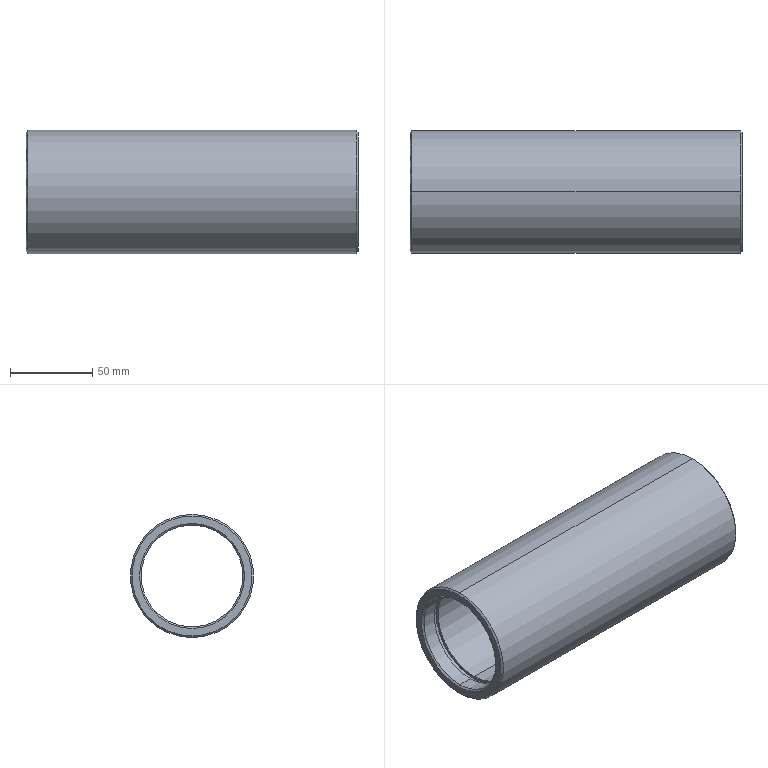Part | SolidWorks | features Chamfer 2, Revolution 1 | 1 solid | 30 faces | box 202 x 75 x 75 mm | volume 280318 mm3 | cone 12 | cylinder 12 | plane 6 | commonest cylinder face diameters 62 x6 65 x4 75 x2
STEP:
#1=CARTESIAN_POINT('',(9.126,0.,-31.));
#2=VERTEX_POINT('',#1);
#3=CARTESIAN_POINT('',(9.126,0.,31.));
#4=VERTEX_POINT('',#3);
#5=CARTESIAN_POINT('',(9.126,0.,0.));
#6=DIRECTION('',(-1.,0.,0.));
#7=DIRECTION('',(0.,0.,-1.));
#8=AXIS2_PLACEMENT_3D('',#5,#6,#7);
#9=CIRCLE('',#8,31.);
#10=EDGE_CURVE('',#2,#4,#9,.T.);
#11=ORIENTED_EDGE('',*,*,#10,.F.);
#12=CARTESIAN_POINT('',(8.876,0.,-31.25));
#13=VERTEX_POINT('',#12);
#14=CARTESIAN_POINT('',(9.126,0.,-31.));
#15=DIRECTION('',(-0.7071,0.,-0.7071));
#16=VECTOR('',#15,1000.);
#17=LINE('',#14,#16);
#18=EDGE_CURVE('',#2,#13,#17,.T.);
#19=ORIENTED_EDGE('',*,*,#18,.T.);
#20=CARTESIAN_POINT('',(8.876,0.,31.25));
#21=VERTEX_POINT('',#20);
#22=CARTESIAN_POINT('',(8.876,0.,0.));
#23=DIRECTION('',(1.,0.,0.));
#24=DIRECTION('',(0.,0.,-1.));
#25=AXIS2_PLACEMENT_3D('',#22,#23,#24);
#26=CIRCLE('',#25,31.25);
#27=EDGE_CURVE('',#21,#13,#26,.T.);
#28=ORIENTED_EDGE('',*,*,#27,.F.);
#29=CARTESIAN_POINT('',(9.126,0.,31.));
#30=DIRECTION('',(-0.7071,0.,0.7071));
#31=VECTOR('',#30,1000.);
#32=LINE('',#29,#31);
#33=EDGE_CURVE('',#4,#21,#32,.T.);
#34=ORIENTED_EDGE('',*,*,#33,.F.);
#35=EDGE_LOOP('',(#11,#19,#28,#34));
#36=FACE_OUTER_BOUND('',#35,.T.);
#37=CARTESIAN_POINT('',(9.126,0.,0.));
#38=DIRECTION('',(-1.,0.,0.));
#39=DIRECTION('',(0.,0.,1.));
#40=AXIS2_PLACEMENT_3D('',#37,#38,#39);
#41=CONICAL_SURFACE('',#40,31.,0.7854);
#42=ADVANCED_FACE('',(#36),#41,.F.);
#43=CARTESIAN_POINT('',(184.626,0.,31.));
#44=VERTEX_POINT('',#43);
#45=CARTESIAN_POINT('',(184.626,0.,-31.));
#46=VERTEX_POINT('',#45);
#47=CARTESIAN_POINT('',(184.626,0.,0.));
#48=DIRECTION('',(1.,0.,0.));
#49=DIRECTION('',(0.,0.,1.));
#50=AXIS2_PLACEMENT_3D('',#47,#48,#49);
#51=CIRCLE('',#50,31.);
#52=EDGE_CURVE('',#44,#46,#51,.T.);
#53=ORIENTED_EDGE('',*,*,#52,.F.);
#54=CARTESIAN_POINT('',(184.876,0.,31.25));
#55=VERTEX_POINT('',#54);
#56=CARTESIAN_POINT('',(184.876,0.,31.25));
#57=DIRECTION('',(0.7071,0.,0.7071));
#58=VECTOR('',#57,1000.);
#59=LINE('',#56,#58);
#60=EDGE_CURVE('',#44,#55,#59,.T.);
#61=ORIENTED_EDGE('',*,*,#60,.T.);
#62=CARTESIAN_POINT('',(184.876,0.,-31.25));
#63=VERTEX_POINT('',#62);
#64=CARTESIAN_POINT('',(184.876,0.,0.));
#65=DIRECTION('',(-1.,0.,0.));
#66=DIRECTION('',(0.,0.,1.));
#67=AXIS2_PLACEMENT_3D('',#64,#65,#66);
#68=CIRCLE('',#67,31.25);
#69=EDGE_CURVE('',#63,#55,#68,.T.);
#70=ORIENTED_EDGE('',*,*,#69,.F.);
#71=CARTESIAN_POINT('',(184.876,0.,-31.25));
#72=DIRECTION('',(0.7071,0.,-0.7071));
#73=VECTOR('',#72,1000.);
#74=LINE('',#71,#73);
#75=EDGE_CURVE('',#46,#63,#74,.T.);
#76=ORIENTED_EDGE('',*,*,#75,.F.);
#77=EDGE_LOOP('',(#53,#61,#70,#76));
#78=FACE_OUTER_BOUND('',#77,.T.);
#79=CARTESIAN_POINT('',(184.876,0.,0.));
#80=DIRECTION('',(1.,0.,0.));
#81=DIRECTION('',(0.,0.,-1.));
#82=AXIS2_PLACEMENT_3D('',#79,#80,#81);
#83=CONICAL_SURFACE('',#82,31.25,0.7854);
#84=ADVANCED_FACE('',(#78),#83,.F.);
#85=CARTESIAN_POINT('',(196.876,0.,31.));
#86=VERTEX_POINT('',#85);
#87=CARTESIAN_POINT('',(196.876,0.,-31.));
#88=VERTEX_POINT('',#87);
#89=CARTESIAN_POINT('',(196.876,0.,0.));
#90=DIRECTION('',(1.,0.,0.));
#91=DIRECTION('',(0.,0.,1.));
#92=AXIS2_PLACEMENT_3D('',#89,#90,#91);
#93=CIRCLE('',#92,31.);
#94=EDGE_CURVE('',#86,#88,#93,.T.);
#95=ORIENTED_EDGE('',*,*,#94,.F.);
#96=CARTESIAN_POINT('',(197.876,0.,32.));
#97=VERTEX_POINT('',#96);
#98=CARTESIAN_POINT('',(197.876,0.,32.));
#99=DIRECTION('',(0.7071,0.,0.7071));
#100=VECTOR('',#99,1000.);
#101=LINE('',#98,#100);
#102=EDGE_CURVE('',#86,#97,#101,.T.);
#103=ORIENTED_EDGE('',*,*,#102,.T.);
#104=CARTESIAN_POINT('',(197.876,0.,-32.));
#105=VERTEX_POINT('',#104);
#106=CARTESIAN_POINT('',(197.876,0.,0.));
#107=DIRECTION('',(-1.,0.,0.));
#108=DIRECTION('',(0.,0.,1.));
#109=AXIS2_PLACEMENT_3D('',#106,#107,#108);
#110=CIRCLE('',#109,32.);
#111=EDGE_CURVE('',#105,#97,#110,.T.);
#112=ORIENTED_EDGE('',*,*,#111,.F.);
#113=CARTESIAN_POINT('',(197.876,0.,-32.));
#114=DIRECTION('',(0.7071,0.,-0.7071));
#115=VECTOR('',#114,1000.);
#116=LINE('',#113,#115);
#117=EDGE_CURVE('',#88,#105,#116,.T.);
#118=ORIENTED_EDGE('',*,*,#117,.F.);
#119=EDGE_LOOP('',(#95,#103,#112,#118));
#120=FACE_OUTER_BOUND('',#119,.T.);
#121=CARTESIAN_POINT('',(197.876,0.,0.));
#122=DIRECTION('',(1.,0.,0.));
#123=DIRECTION('',(0.,0.,-1.));
#124=AXIS2_PLACEMENT_3D('',#121,#122,#123);
#125=CONICAL_SURFACE('',#124,32.,0.7854);
#126=ADVANCED_FACE('',(#120),#125,.F.);
#127=CARTESIAN_POINT('',(197.876,0.,-36.5));
#128=VERTEX_POINT('',#127);
#129=CARTESIAN_POINT('',(197.876,0.,36.5));
#130=VERTEX_POINT('',#129);
#131=CARTESIAN_POINT('',(197.876,0.,0.));
#132=DIRECTION('',(1.,0.,0.));
#133=DIRECTION('',(0.,0.,1.));
#134=AXIS2_PLACEMENT_3D('',#131,#132,#133);
#135=CIRCLE('',#134,36.5);
#136=EDGE_CURVE('',#128,#130,#135,.T.);
#137=ORIENTED_EDGE('',*,*,#136,.F.);
#138=CARTESIAN_POINT('',(196.876,0.,-37.5));
#139=VERTEX_POINT('',#138);
#140=CARTESIAN_POINT('',(196.876,0.,-37.5));
#141=DIRECTION('',(-0.7071,0.,-0.7071));
#142=VECTOR('',#141,1000.);
#143=LINE('',#140,#142);
#144=EDGE_CURVE('',#128,#139,#143,.T.);
#145=ORIENTED_EDGE('',*,*,#144,.T.);
#146=CARTESIAN_POINT('',(196.876,0.,37.5));
#147=VERTEX_POINT('',#146);
#148=CARTESIAN_POINT('',(196.876,0.,0.));
#149=DIRECTION('',(-1.,0.,0.));
#150=DIRECTION('',(0.,0.,1.));
#151=AXIS2_PLACEMENT_3D('',#148,#149,#150);
#152=CIRCLE('',#151,37.5);
#153=EDGE_CURVE('',#147,#139,#152,.T.);
#154=ORIENTED_EDGE('',*,*,#153,.F.);
#155=CARTESIAN_POINT('',(196.876,0.,37.5));
#156=DIRECTION('',(-0.7071,0.,0.7071));
#157=VECTOR('',#156,1000.);
#158=LINE('',#155,#157);
#159=EDGE_CURVE('',#130,#147,#158,.T.);
#160=ORIENTED_EDGE('',*,*,#159,.F.);
#161=EDGE_LOOP('',(#137,#145,#154,#160));
#162=FACE_OUTER_BOUND('',#161,.T.);
#163=CARTESIAN_POINT('',(196.876,0.,0.));
#164=DIRECTION('',(-1.,0.,0.));
#165=DIRECTION('',(0.,0.,1.));
#166=AXIS2_PLACEMENT_3D('',#163,#164,#165);
#167=CONICAL_SURFACE('',#166,37.5,0.7854);
#168=ADVANCED_FACE('',(#162),#167,.T.);
#169=CARTESIAN_POINT('',(-3.124,0.,-31.));
#170=VERTEX_POINT('',#169);
#171=CARTESIAN_POINT('',(-3.124,0.,31.));
#172=VERTEX_POINT('',#171);
#173=CARTESIAN_POINT('',(-3.124,0.,0.));
#174=DIRECTION('',(-1.,0.,0.));
#175=DIRECTION('',(0.,0.,-1.));
#176=AXIS2_PLACEMENT_3D('',#173,#174,#175);
#177=CIRCLE('',#176,31.);
#178=EDGE_CURVE('',#170,#172,#177,.T.);
#179=ORIENTED_EDGE('',*,*,#178,.F.);
#180=CARTESIAN_POINT('',(-4.124,0.,-32.));
#181=VERTEX_POINT('',#180);
#182=CARTESIAN_POINT('',(-3.124,0.,-31.));
#183=DIRECTION('',(-0.7071,0.,-0.7071));
#184=VECTOR('',#183,1000.);
#185=LINE('',#182,#184);
#186=EDGE_CURVE('',#170,#181,#185,.T.);
#187=ORIENTED_EDGE('',*,*,#186,.T.);
#188=CARTESIAN_POINT('',(-4.124,0.,32.));
#189=VERTEX_POINT('',#188);
#190=CARTESIAN_POINT('',(-4.124,0.,0.));
#191=DIRECTION('',(1.,0.,0.));
#192=DIRECTION('',(0.,0.,-1.));
#193=AXIS2_PLACEMENT_3D('',#190,#191,#192);
#194=CIRCLE('',#193,32.);
#195=EDGE_CURVE('',#189,#181,#194,.T.);
#196=ORIENTED_EDGE('',*,*,#195,.F.);
#197=CARTESIAN_POINT('',(-3.124,0.,31.));
#198=DIRECTION('',(-0.7071,0.,0.7071));
#199=VECTOR('',#198,1000.);
#200=LINE('',#197,#199);
#201=EDGE_CURVE('',#172,#189,#200,.T.);
#202=ORIENTED_EDGE('',*,*,#201,.F.);
#203=EDGE_LOOP('',(#179,#187,#196,#202));
#204=FACE_OUTER_BOUND('',#203,.T.);
#205=CARTESIAN_POINT('',(-3.124,0.,0.));
#206=DIRECTION('',(-1.,0.,0.));
#207=DIRECTION('',(0.,0.,1.));
#208=AXIS2_PLACEMENT_3D('',#205,#206,#207);
#209=CONICAL_SURFACE('',#208,31.,0.7854);
#210=ADVANCED_FACE('',(#204),#209,.F.);
#211=CARTESIAN_POINT('',(-4.124,0.,36.5));
#212=VERTEX_POINT('',#211);
#213=CARTESIAN_POINT('',(-4.124,0.,-36.5));
#214=VERTEX_POINT('',#213);
#215=CARTESIAN_POINT('',(-4.124,0.,0.));
#216=DIRECTION('',(-1.,0.,0.));
#217=DIRECTION('',(0.,0.,-1.));
#218=AXIS2_PLACEMENT_3D('',#215,#216,#217);
#219=CIRCLE('',#218,36.5);
#220=EDGE_CURVE('',#212,#214,#219,.T.);
#221=ORIENTED_EDGE('',*,*,#220,.F.);
#222=CARTESIAN_POINT('',(-3.124,0.,37.5));
#223=VERTEX_POINT('',#222);
#224=CARTESIAN_POINT('',(-4.124,0.,36.5));
#225=DIRECTION('',(0.7071,0.,0.7071));
#226=VECTOR('',#225,1000.);
#227=LINE('',#224,#226);
#228=EDGE_CURVE('',#212,#223,#227,.T.);
#229=ORIENTED_EDGE('',*,*,#228,.T.);
#230=CARTESIAN_POINT('',(-3.124,0.,-37.5));
#231=VERTEX_POINT('',#230);
#232=CARTESIAN_POINT('',(-3.124,0.,0.));
#233=DIRECTION('',(1.,0.,0.));
#234=DIRECTION('',(0.,0.,-1.));
#235=AXIS2_PLACEMENT_3D('',#232,#233,#234);
#236=CIRCLE('',#235,37.5);
#237=EDGE_CURVE('',#231,#223,#236,.T.);
#238=ORIENTED_EDGE('',*,*,#237,.F.);
#239=CARTESIAN_POINT('',(-4.124,0.,-36.5));
#240=DIRECTION('',(0.7071,0.,-0.7071));
#241=VECTOR('',#240,1000.);
#242=LINE('',#239,#241);
#243=EDGE_CURVE('',#214,#231,#242,.T.);
#244=ORIENTED_EDGE('',*,*,#243,.F.);
#245=EDGE_LOOP('',(#221,#229,#238,#244));
#246=FACE_OUTER_BOUND('',#245,.T.);
#247=CARTESIAN_POINT('',(-4.124,0.,0.));
#248=DIRECTION('',(1.,0.,0.));
#249=DIRECTION('',(0.,0.,-1.));
#250=AXIS2_PLACEMENT_3D('',#247,#248,#249);
#251=CONICAL_SURFACE('',#250,36.5,0.7854);
#252=ADVANCED_FACE('',(#246),#251,.T.);
#253=CARTESIAN_POINT('',(5.876,0.,-31.));
#254=VERTEX_POINT('',#253);
#255=CARTESIAN_POINT('',(5.876,0.,31.));
#256=VERTEX_POINT('',#255);
#257=CARTESIAN_POINT('',(5.876,0.,0.));
#258=DIRECTION('',(-1.,0.,0.));
#259=DIRECTION('',(0.,0.,1.));
#260=AXIS2_PLACEMENT_3D('',#257,#258,#259);
#261=CIRCLE('',#260,31.);
#262=EDGE_CURVE('',#254,#256,#261,.T.);
#263=ORIENTED_EDGE('',*,*,#262,.F.);
#264=CARTESIAN_POINT('',(0.,0.,-31.));
#265=DIRECTION('',(-1.,0.,0.));
#266=VECTOR('',#265,1000.);
#267=LINE('',#264,#266);
#268=EDGE_CURVE('',#254,#170,#267,.T.);
#269=ORIENTED_EDGE('',*,*,#268,.T.);
#270=ORIENTED_EDGE('',*,*,#178,.T.);
#271=CARTESIAN_POINT('',(0.,0.,31.));
#272=DIRECTION('',(-1.,0.,0.));
#273=VECTOR('',#272,1000.);
#274=LINE('',#271,#273);
#275=EDGE_CURVE('',#256,#172,#274,.T.);
#276=ORIENTED_EDGE('',*,*,#275,.F.);
#277=EDGE_LOOP('',(#263,#269,#270,#276));
#278=FACE_OUTER_BOUND('',#277,.T.);
#279=CARTESIAN_POINT('',(0.,0.,0.));
#280=DIRECTION('',(-1.,0.,0.));
#281=DIRECTION('',(0.,0.,1.));
#282=AXIS2_PLACEMENT_3D('',#279,#280,#281);
#283=CYLINDRICAL_SURFACE('',#282,31.);
#284=ADVANCED_FACE('',(#278),#283,.F.);
#285=CARTESIAN_POINT('',(8.876,0.,-32.5));
#286=VERTEX_POINT('',#285);
#287=CARTESIAN_POINT('',(8.876,0.,32.5));
#288=VERTEX_POINT('',#287);
#289=CARTESIAN_POINT('',(8.876,0.,0.));
#290=DIRECTION('',(-1.,0.,0.));
#291=DIRECTION('',(0.,0.,1.));
#292=AXIS2_PLACEMENT_3D('',#289,#290,#291);
#293=CIRCLE('',#292,32.5);
#294=EDGE_CURVE('',#286,#288,#293,.T.);
#295=ORIENTED_EDGE('',*,*,#294,.F.);
#296=CARTESIAN_POINT('',(5.876,0.,-32.5));
#297=VERTEX_POINT('',#296);
#298=CARTESIAN_POINT('',(0.,0.,-32.5));
#299=DIRECTION('',(-1.,0.,0.));
#300=VECTOR('',#299,1000.);
#301=LINE('',#298,#300);
#302=EDGE_CURVE('',#286,#297,#301,.T.);
#303=ORIENTED_EDGE('',*,*,#302,.T.);
#304=CARTESIAN_POINT('',(5.876,0.,32.5));
#305=VERTEX_POINT('',#304);
#306=CARTESIAN_POINT('',(5.876,0.,0.));
#307=DIRECTION('',(-1.,0.,0.));
#308=DIRECTION('',(0.,0.,1.));
#309=AXIS2_PLACEMENT_3D('',#306,#307,#308);
#310=CIRCLE('',#309,32.5);
#311=EDGE_CURVE('',#297,#305,#310,.T.);
#312=ORIENTED_EDGE('',*,*,#311,.T.);
#313=CARTESIAN_POINT('',(0.,0.,32.5));
#314=DIRECTION('',(-1.,0.,0.));
#315=VECTOR('',#314,1000.);
#316=LINE('',#313,#315);
#317=EDGE_CURVE('',#288,#305,#316,.T.);
#318=ORIENTED_EDGE('',*,*,#317,.F.);
#319=EDGE_LOOP('',(#295,#303,#312,#318));
#320=FACE_OUTER_BOUND('',#319,.T.);
#321=CARTESIAN_POINT('',(0.,0.,0.));
#322=DIRECTION('',(-1.,0.,0.));
#323=DIRECTION('',(0.,0.,1.));
#324=AXIS2_PLACEMENT_3D('',#321,#322,#323);
#325=CYLINDRICAL_SURFACE('',#324,32.5);
#326=ADVANCED_FACE('',(#320),#325,.F.);
#327=ORIENTED_EDGE('',*,*,#52,.T.);
#328=CARTESIAN_POINT('',(0.,0.,-31.));
#329=DIRECTION('',(-1.,0.,0.));
#330=VECTOR('',#329,1000.);
#331=LINE('',#328,#330);
#332=EDGE_CURVE('',#46,#2,#331,.T.);
#333=ORIENTED_EDGE('',*,*,#332,.T.);
#334=ORIENTED_EDGE('',*,*,#10,.T.);
#335=CARTESIAN_POINT('',(0.,0.,31.));
#336=DIRECTION('',(-1.,0.,0.));
#337=VECTOR('',#336,1000.);
#338=LINE('',#335,#337);
#339=EDGE_CURVE('',#44,#4,#338,.T.);
#340=ORIENTED_EDGE('',*,*,#339,.F.);
#341=EDGE_LOOP('',(#327,#333,#334,#340));
#342=FACE_OUTER_BOUND('',#341,.T.);
#343=CARTESIAN_POINT('',(0.,0.,0.));
#344=DIRECTION('',(-1.,0.,0.));
#345=DIRECTION('',(0.,0.,1.));
#346=AXIS2_PLACEMENT_3D('',#343,#344,#345);
#347=CYLINDRICAL_SURFACE('',#346,31.);
#348=ADVANCED_FACE('',(#342),#347,.F.);
#349=CARTESIAN_POINT('',(187.876,0.,-32.5));
#350=VERTEX_POINT('',#349);
#351=CARTESIAN_POINT('',(187.876,0.,32.5));
#352=VERTEX_POINT('',#351);
#353=CARTESIAN_POINT('',(187.876,0.,0.));
#354=DIRECTION('',(-1.,0.,0.));
#355=DIRECTION('',(0.,0.,1.));
#356=AXIS2_PLACEMENT_3D('',#353,#354,#355);
#357=CIRCLE('',#356,32.5);
#358=EDGE_CURVE('',#350,#352,#357,.T.);
#359=ORIENTED_EDGE('',*,*,#358,.F.);
#360=CARTESIAN_POINT('',(184.876,0.,-32.5));
#361=VERTEX_POINT('',#360);
#362=CARTESIAN_POINT('',(0.,0.,-32.5));
#363=DIRECTION('',(-1.,0.,0.));
#364=VECTOR('',#363,1000.);
#365=LINE('',#362,#364);
#366=EDGE_CURVE('',#350,#361,#365,.T.);
#367=ORIENTED_EDGE('',*,*,#366,.T.);
#368=CARTESIAN_POINT('',(184.876,0.,32.5));
#369=VERTEX_POINT('',#368);
#370=CARTESIAN_POINT('',(184.876,0.,0.));
#371=DIRECTION('',(-1.,0.,0.));
#372=DIRECTION('',(0.,0.,1.));
#373=AXIS2_PLACEMENT_3D('',#370,#371,#372);
#374=CIRCLE('',#373,32.5);
#375=EDGE_CURVE('',#361,#369,#374,.T.);
#376=ORIENTED_EDGE('',*,*,#375,.T.);
#377=CARTESIAN_POINT('',(0.,0.,32.5));
#378=DIRECTION('',(-1.,0.,0.));
#379=VECTOR('',#378,1000.);
#380=LINE('',#377,#379);
#381=EDGE_CURVE('',#352,#369,#380,.T.);
#382=ORIENTED_EDGE('',*,*,#381,.F.);
#383=EDGE_LOOP('',(#359,#367,#376,#382));
#384=FACE_OUTER_BOUND('',#383,.T.);
#385=CARTESIAN_POINT('',(0.,0.,0.));
#386=DIRECTION('',(-1.,0.,0.));
#387=DIRECTION('',(0.,0.,1.));
#388=AXIS2_PLACEMENT_3D('',#385,#386,#387);
#389=CYLINDRICAL_SURFACE('',#388,32.5);
#390=ADVANCED_FACE('',(#384),#389,.F.);
#391=ORIENTED_EDGE('',*,*,#94,.T.);
#392=CARTESIAN_POINT('',(187.876,0.,-31.));
#393=VERTEX_POINT('',#392);
#394=CARTESIAN_POINT('',(0.,0.,-31.));
#395=DIRECTION('',(-1.,0.,0.));
#396=VECTOR('',#395,1000.);
#397=LINE('',#394,#396);
#398=EDGE_CURVE('',#88,#393,#397,.T.);
#399=ORIENTED_EDGE('',*,*,#398,.T.);
#400=CARTESIAN_POINT('',(187.876,0.,31.));
#401=VERTEX_POINT('',#400);
#402=CARTESIAN_POINT('',(187.876,0.,0.));
#403=DIRECTION('',(-1.,0.,0.));
#404=DIRECTION('',(0.,0.,1.));
#405=AXIS2_PLACEMENT_3D('',#402,#403,#404);
#406=CIRCLE('',#405,31.);
#407=EDGE_CURVE('',#393,#401,#406,.T.);
#408=ORIENTED_EDGE('',*,*,#407,.T.);
#409=CARTESIAN_POINT('',(0.,0.,31.));
#410=DIRECTION('',(-1.,0.,0.));
#411=VECTOR('',#410,1000.);
#412=LINE('',#409,#411);
#413=EDGE_CURVE('',#86,#401,#412,.T.);
#414=ORIENTED_EDGE('',*,*,#413,.F.);
#415=EDGE_LOOP('',(#391,#399,#408,#414));
#416=FACE_OUTER_BOUND('',#415,.T.);
#417=CARTESIAN_POINT('',(0.,0.,0.));
#418=DIRECTION('',(-1.,0.,0.));
#419=DIRECTION('',(0.,0.,1.));
#420=AXIS2_PLACEMENT_3D('',#417,#418,#419);
#421=CYLINDRICAL_SURFACE('',#420,31.);
#422=ADVANCED_FACE('',(#416),#421,.F.);
#423=ORIENTED_EDGE('',*,*,#153,.T.);
#424=CARTESIAN_POINT('',(0.,0.,-37.5));
#425=DIRECTION('',(-1.,0.,0.));
#426=VECTOR('',#425,1000.);
#427=LINE('',#424,#426);
#428=EDGE_CURVE('',#139,#231,#427,.T.);
#429=ORIENTED_EDGE('',*,*,#428,.T.);
#430=ORIENTED_EDGE('',*,*,#237,.T.);
#431=CARTESIAN_POINT('',(0.,0.,37.5));
#432=DIRECTION('',(-1.,0.,0.));
#433=VECTOR('',#432,1000.);
#434=LINE('',#431,#433);
#435=EDGE_CURVE('',#147,#223,#434,.T.);
#436=ORIENTED_EDGE('',*,*,#435,.F.);
#437=EDGE_LOOP('',(#423,#429,#430,#436));
#438=FACE_OUTER_BOUND('',#437,.T.);
#439=CARTESIAN_POINT('',(0.,0.,0.));
#440=DIRECTION('',(-1.,0.,0.));
#441=DIRECTION('',(0.,0.,1.));
#442=AXIS2_PLACEMENT_3D('',#439,#440,#441);
#443=CYLINDRICAL_SURFACE('',#442,37.5);
#444=ADVANCED_FACE('',(#438),#443,.T.);
#445=CARTESIAN_POINT('',(-4.124,0.,0.));
#446=DIRECTION('',(-1.,0.,0.));
#447=DIRECTION('',(0.,0.,-1.));
#448=AXIS2_PLACEMENT_3D('',#445,#446,#447);
#449=CIRCLE('',#448,36.5);
#450=EDGE_CURVE('',#214,#212,#449,.T.);
#451=ORIENTED_EDGE('',*,*,#450,.T.);
#452=ORIENTED_EDGE('',*,*,#220,.T.);
#453=EDGE_LOOP('',(#451,#452));
#454=FACE_OUTER_BOUND('',#453,.T.);
#455=ORIENTED_EDGE('',*,*,#195,.T.);
#456=CARTESIAN_POINT('',(-4.124,0.,0.));
#457=DIRECTION('',(1.,0.,0.));
#458=DIRECTION('',(0.,0.,-1.));
#459=AXIS2_PLACEMENT_3D('',#456,#457,#458);
#460=CIRCLE('',#459,32.);
#461=EDGE_CURVE('',#181,#189,#460,.T.);
#462=ORIENTED_EDGE('',*,*,#461,.T.);
#463=EDGE_LOOP('',(#455,#462));
#464=FACE_BOUND('',#463,.T.);
#465=CARTESIAN_POINT('',(-4.124,31.,0.));
#466=DIRECTION('',(1.,0.,0.));
#467=DIRECTION('',(0.,0.,-1.));
#468=AXIS2_PLACEMENT_3D('',#465,#466,#467);
#469=PLANE('',#468);
#470=ADVANCED_FACE('',(#454,#464),#469,.F.);
#471=ORIENTED_EDGE('',*,*,#428,.F.);
#472=CARTESIAN_POINT('',(196.876,0.,0.));
#473=DIRECTION('',(-1.,0.,0.));
#474=DIRECTION('',(0.,0.,1.));
#475=AXIS2_PLACEMENT_3D('',#472,#473,#474);
#476=CIRCLE('',#475,37.5);
#477=EDGE_CURVE('',#139,#147,#476,.T.);
#478=ORIENTED_EDGE('',*,*,#477,.T.);
#479=ORIENTED_EDGE('',*,*,#435,.T.);
#480=CARTESIAN_POINT('',(-3.124,0.,0.));
#481=DIRECTION('',(1.,0.,0.));
#482=DIRECTION('',(0.,0.,-1.));
#483=AXIS2_PLACEMENT_3D('',#480,#481,#482);
#484=CIRCLE('',#483,37.5);
#485=EDGE_CURVE('',#223,#231,#484,.T.);
#486=ORIENTED_EDGE('',*,*,#485,.T.);
#487=EDGE_LOOP('',(#471,#478,#479,#486));
#488=FACE_OUTER_BOUND('',#487,.T.);
#489=CARTESIAN_POINT('',(0.,0.,0.));
#490=DIRECTION('',(-1.,0.,0.));
#491=DIRECTION('',(0.,0.,1.));
#492=AXIS2_PLACEMENT_3D('',#489,#490,#491);
#493=CYLINDRICAL_SURFACE('',#492,37.5);
#494=ADVANCED_FACE('',(#488),#493,.T.);
#495=CARTESIAN_POINT('',(197.876,0.,0.));
#496=DIRECTION('',(1.,0.,0.));
#497=DIRECTION('',(0.,0.,1.));
#498=AXIS2_PLACEMENT_3D('',#495,#496,#497);
#499=CIRCLE('',#498,36.5);
#500=EDGE_CURVE('',#130,#128,#499,.T.);
#501=ORIENTED_EDGE('',*,*,#500,.T.);
#502=ORIENTED_EDGE('',*,*,#136,.T.);
#503=EDGE_LOOP('',(#501,#502));
#504=FACE_OUTER_BOUND('',#503,.T.);
#505=ORIENTED_EDGE('',*,*,#111,.T.);
#506=CARTESIAN_POINT('',(197.876,0.,0.));
#507=DIRECTION('',(-1.,0.,0.));
#508=DIRECTION('',(0.,0.,1.));
#509=AXIS2_PLACEMENT_3D('',#506,#507,#508);
#510=CIRCLE('',#509,32.);
#511=EDGE_CURVE('',#97,#105,#510,.T.);
#512=ORIENTED_EDGE('',*,*,#511,.T.);
#513=EDGE_LOOP('',(#505,#512));
#514=FACE_BOUND('',#513,.T.);
#515=CARTESIAN_POINT('',(197.876,37.5,0.));
#516=DIRECTION('',(-1.,0.,0.));
#517=DIRECTION('',(0.,0.,1.));
#518=AXIS2_PLACEMENT_3D('',#515,#516,#517);
#519=PLANE('',#518);
#520=ADVANCED_FACE('',(#504,#514),#519,.F.);
#521=ORIENTED_EDGE('',*,*,#398,.F.);
#522=CARTESIAN_POINT('',(196.876,0.,0.));
#523=DIRECTION('',(1.,0.,0.));
#524=DIRECTION('',(0.,0.,1.));
#525=AXIS2_PLACEMENT_3D('',#522,#523,#524);
#526=CIRCLE('',#525,31.);
#527=EDGE_CURVE('',#88,#86,#526,.T.);
#528=ORIENTED_EDGE('',*,*,#527,.T.);
#529=ORIENTED_EDGE('',*,*,#413,.T.);
#530=CARTESIAN_POINT('',(187.876,0.,0.));
#531=DIRECTION('',(-1.,0.,0.));
#532=DIRECTION('',(0.,0.,1.));
#533=AXIS2_PLACEMENT_3D('',#530,#531,#532);
#534=CIRCLE('',#533,31.);
#535=EDGE_CURVE('',#401,#393,#534,.T.);
#536=ORIENTED_EDGE('',*,*,#535,.T.);
#537=EDGE_LOOP('',(#521,#528,#529,#536));
#538=FACE_OUTER_BOUND('',#537,.T.);
#539=CARTESIAN_POINT('',(0.,0.,0.));
#540=DIRECTION('',(-1.,0.,0.));
#541=DIRECTION('',(0.,0.,1.));
#542=AXIS2_PLACEMENT_3D('',#539,#540,#541);
#543=CYLINDRICAL_SURFACE('',#542,31.);
#544=ADVANCED_FACE('',(#538),#543,.F.);
#545=ORIENTED_EDGE('',*,*,#535,.F.);
#546=ORIENTED_EDGE('',*,*,#407,.F.);
#547=EDGE_LOOP('',(#545,#546));
#548=FACE_BOUND('',#547,.T.);
#549=CARTESIAN_POINT('',(187.876,0.,0.));
#550=DIRECTION('',(-1.,0.,0.));
#551=DIRECTION('',(0.,0.,1.));
#552=AXIS2_PLACEMENT_3D('',#549,#550,#551);
#553=CIRCLE('',#552,32.5);
#554=EDGE_CURVE('',#352,#350,#553,.T.);
#555=ORIENTED_EDGE('',*,*,#554,.T.);
#556=ORIENTED_EDGE('',*,*,#358,.T.);
#557=EDGE_LOOP('',(#555,#556));
#558=FACE_OUTER_BOUND('',#557,.T.);
#559=CARTESIAN_POINT('',(187.876,31.,0.));
#560=DIRECTION('',(1.,0.,0.));
#561=DIRECTION('',(0.,0.,-1.));
#562=AXIS2_PLACEMENT_3D('',#559,#560,#561);
#563=PLANE('',#562);
#564=ADVANCED_FACE('',(#548,#558),#563,.F.);
#565=ORIENTED_EDGE('',*,*,#366,.F.);
#566=ORIENTED_EDGE('',*,*,#554,.F.);
#567=ORIENTED_EDGE('',*,*,#381,.T.);
#568=CARTESIAN_POINT('',(184.876,0.,0.));
#569=DIRECTION('',(-1.,0.,0.));
#570=DIRECTION('',(0.,0.,1.));
#571=AXIS2_PLACEMENT_3D('',#568,#569,#570);
#572=CIRCLE('',#571,32.5);
#573=EDGE_CURVE('',#369,#361,#572,.T.);
#574=ORIENTED_EDGE('',*,*,#573,.T.);
#575=EDGE_LOOP('',(#565,#566,#567,#574));
#576=FACE_OUTER_BOUND('',#575,.T.);
#577=CARTESIAN_POINT('',(0.,0.,0.));
#578=DIRECTION('',(-1.,0.,0.));
#579=DIRECTION('',(0.,0.,1.));
#580=AXIS2_PLACEMENT_3D('',#577,#578,#579);
#581=CYLINDRICAL_SURFACE('',#580,32.5);
#582=ADVANCED_FACE('',(#576),#581,.F.);
#583=ORIENTED_EDGE('',*,*,#69,.T.);
#584=CARTESIAN_POINT('',(184.876,0.,0.));
#585=DIRECTION('',(-1.,0.,0.));
#586=DIRECTION('',(0.,0.,1.));
#587=AXIS2_PLACEMENT_3D('',#584,#585,#586);
#588=CIRCLE('',#587,31.25);
#589=EDGE_CURVE('',#55,#63,#588,.T.);
#590=ORIENTED_EDGE('',*,*,#589,.T.);
#591=EDGE_LOOP('',(#583,#590));
#592=FACE_BOUND('',#591,.T.);
#593=ORIENTED_EDGE('',*,*,#573,.F.);
#594=ORIENTED_EDGE('',*,*,#375,.F.);
#595=EDGE_LOOP('',(#593,#594));
#596=FACE_OUTER_BOUND('',#595,.T.);
#597=CARTESIAN_POINT('',(184.876,32.5,0.));
#598=DIRECTION('',(-1.,0.,0.));
#599=DIRECTION('',(0.,0.,1.));
#600=AXIS2_PLACEMENT_3D('',#597,#598,#599);
#601=PLANE('',#600);
#602=ADVANCED_FACE('',(#592,#596),#601,.F.);
#603=ORIENTED_EDGE('',*,*,#332,.F.);
#604=CARTESIAN_POINT('',(184.626,0.,0.));
#605=DIRECTION('',(1.,0.,0.));
#606=DIRECTION('',(0.,0.,1.));
#607=AXIS2_PLACEMENT_3D('',#604,#605,#606);
#608=CIRCLE('',#607,31.);
#609=EDGE_CURVE('',#46,#44,#608,.T.);
#610=ORIENTED_EDGE('',*,*,#609,.T.);
#611=ORIENTED_EDGE('',*,*,#339,.T.);
#612=CARTESIAN_POINT('',(9.126,0.,0.));
#613=DIRECTION('',(-1.,0.,0.));
#614=DIRECTION('',(0.,0.,-1.));
#615=AXIS2_PLACEMENT_3D('',#612,#613,#614);
#616=CIRCLE('',#615,31.);
#617=EDGE_CURVE('',#4,#2,#616,.T.);
#618=ORIENTED_EDGE('',*,*,#617,.T.);
#619=EDGE_LOOP('',(#603,#610,#611,#618));
#620=FACE_OUTER_BOUND('',#619,.T.);
#621=CARTESIAN_POINT('',(0.,0.,0.));
#622=DIRECTION('',(-1.,0.,0.));
#623=DIRECTION('',(0.,0.,1.));
#624=AXIS2_PLACEMENT_3D('',#621,#622,#623);
#625=CYLINDRICAL_SURFACE('',#624,31.);
#626=ADVANCED_FACE('',(#620),#625,.F.);
#627=ORIENTED_EDGE('',*,*,#27,.T.);
#628=CARTESIAN_POINT('',(8.876,0.,0.));
#629=DIRECTION('',(1.,0.,0.));
#630=DIRECTION('',(0.,0.,-1.));
#631=AXIS2_PLACEMENT_3D('',#628,#629,#630);
#632=CIRCLE('',#631,31.25);
#633=EDGE_CURVE('',#13,#21,#632,.T.);
#634=ORIENTED_EDGE('',*,*,#633,.T.);
#635=EDGE_LOOP('',(#627,#634));
#636=FACE_BOUND('',#635,.T.);
#637=CARTESIAN_POINT('',(8.876,0.,0.));
#638=DIRECTION('',(-1.,0.,0.));
#639=DIRECTION('',(0.,0.,1.));
#640=AXIS2_PLACEMENT_3D('',#637,#638,#639);
#641=CIRCLE('',#640,32.5);
#642=EDGE_CURVE('',#288,#286,#641,.T.);
#643=ORIENTED_EDGE('',*,*,#642,.T.);
#644=ORIENTED_EDGE('',*,*,#294,.T.);
#645=EDGE_LOOP('',(#643,#644));
#646=FACE_OUTER_BOUND('',#645,.T.);
#647=CARTESIAN_POINT('',(8.876,32.5,0.));
#648=DIRECTION('',(1.,0.,0.));
#649=DIRECTION('',(0.,0.,-1.));
#650=AXIS2_PLACEMENT_3D('',#647,#648,#649);
#651=PLANE('',#650);
#652=ADVANCED_FACE('',(#636,#646),#651,.F.);
#653=ORIENTED_EDGE('',*,*,#302,.F.);
#654=ORIENTED_EDGE('',*,*,#642,.F.);
#655=ORIENTED_EDGE('',*,*,#317,.T.);
#656=CARTESIAN_POINT('',(5.876,0.,0.));
#657=DIRECTION('',(-1.,0.,0.));
#658=DIRECTION('',(0.,0.,1.));
#659=AXIS2_PLACEMENT_3D('',#656,#657,#658);
#660=CIRCLE('',#659,32.5);
#661=EDGE_CURVE('',#305,#297,#660,.T.);
#662=ORIENTED_EDGE('',*,*,#661,.T.);
#663=EDGE_LOOP('',(#653,#654,#655,#662));
#664=FACE_OUTER_BOUND('',#663,.T.);
#665=CARTESIAN_POINT('',(0.,0.,0.));
#666=DIRECTION('',(-1.,0.,0.));
#667=DIRECTION('',(0.,0.,1.));
#668=AXIS2_PLACEMENT_3D('',#665,#666,#667);
#669=CYLINDRICAL_SURFACE('',#668,32.5);
#670=ADVANCED_FACE('',(#664),#669,.F.);
#671=ORIENTED_EDGE('',*,*,#661,.F.);
#672=ORIENTED_EDGE('',*,*,#311,.F.);
#673=EDGE_LOOP('',(#671,#672));
#674=FACE_OUTER_BOUND('',#673,.T.);
#675=CARTESIAN_POINT('',(5.876,0.,0.));
#676=DIRECTION('',(-1.,0.,0.));
#677=DIRECTION('',(0.,0.,1.));
#678=AXIS2_PLACEMENT_3D('',#675,#676,#677);
#679=CIRCLE('',#678,31.);
#680=EDGE_CURVE('',#256,#254,#679,.T.);
#681=ORIENTED_EDGE('',*,*,#680,.T.);
#682=ORIENTED_EDGE('',*,*,#262,.T.);
#683=EDGE_LOOP('',(#681,#682));
#684=FACE_BOUND('',#683,.T.);
#685=CARTESIAN_POINT('',(5.876,31.,0.));
#686=DIRECTION('',(-1.,0.,0.));
#687=DIRECTION('',(0.,0.,1.));
#688=AXIS2_PLACEMENT_3D('',#685,#686,#687);
#689=PLANE('',#688);
#690=ADVANCED_FACE('',(#674,#684),#689,.F.);
#691=ORIENTED_EDGE('',*,*,#268,.F.);
#692=ORIENTED_EDGE('',*,*,#680,.F.);
#693=ORIENTED_EDGE('',*,*,#275,.T.);
#694=CARTESIAN_POINT('',(-3.124,0.,0.));
#695=DIRECTION('',(-1.,0.,0.));
#696=DIRECTION('',(0.,0.,-1.));
#697=AXIS2_PLACEMENT_3D('',#694,#695,#696);
#698=CIRCLE('',#697,31.);
#699=EDGE_CURVE('',#172,#170,#698,.T.);
#700=ORIENTED_EDGE('',*,*,#699,.T.);
#701=EDGE_LOOP('',(#691,#692,#693,#700));
#702=FACE_OUTER_BOUND('',#701,.T.);
#703=CARTESIAN_POINT('',(0.,0.,0.));
#704=DIRECTION('',(-1.,0.,0.));
#705=DIRECTION('',(0.,0.,1.));
#706=AXIS2_PLACEMENT_3D('',#703,#704,#705);
#707=CYLINDRICAL_SURFACE('',#706,31.);
#708=ADVANCED_FACE('',(#702),#707,.F.);
#709=ORIENTED_EDGE('',*,*,#228,.F.);
#710=ORIENTED_EDGE('',*,*,#450,.F.);
#711=ORIENTED_EDGE('',*,*,#243,.T.);
#712=ORIENTED_EDGE('',*,*,#485,.F.);
#713=EDGE_LOOP('',(#709,#710,#711,#712));
#714=FACE_OUTER_BOUND('',#713,.T.);
#715=CARTESIAN_POINT('',(-4.124,0.,0.));
#716=DIRECTION('',(1.,0.,0.));
#717=DIRECTION('',(0.,0.,-1.));
#718=AXIS2_PLACEMENT_3D('',#715,#716,#717);
#719=CONICAL_SURFACE('',#718,36.5,0.7854);
#720=ADVANCED_FACE('',(#714),#719,.T.);
#721=ORIENTED_EDGE('',*,*,#186,.F.);
#722=ORIENTED_EDGE('',*,*,#699,.F.);
#723=ORIENTED_EDGE('',*,*,#201,.T.);
#724=ORIENTED_EDGE('',*,*,#461,.F.);
#725=EDGE_LOOP('',(#721,#722,#723,#724));
#726=FACE_OUTER_BOUND('',#725,.T.);
#727=CARTESIAN_POINT('',(-3.124,0.,0.));
#728=DIRECTION('',(-1.,0.,0.));
#729=DIRECTION('',(0.,0.,1.));
#730=AXIS2_PLACEMENT_3D('',#727,#728,#729);
#731=CONICAL_SURFACE('',#730,31.,0.7854);
#732=ADVANCED_FACE('',(#726),#731,.F.);
#733=ORIENTED_EDGE('',*,*,#144,.F.);
#734=ORIENTED_EDGE('',*,*,#500,.F.);
#735=ORIENTED_EDGE('',*,*,#159,.T.);
#736=ORIENTED_EDGE('',*,*,#477,.F.);
#737=EDGE_LOOP('',(#733,#734,#735,#736));
#738=FACE_OUTER_BOUND('',#737,.T.);
#739=CARTESIAN_POINT('',(196.876,0.,0.));
#740=DIRECTION('',(-1.,0.,0.));
#741=DIRECTION('',(0.,0.,1.));
#742=AXIS2_PLACEMENT_3D('',#739,#740,#741);
#743=CONICAL_SURFACE('',#742,37.5,0.7854);
#744=ADVANCED_FACE('',(#738),#743,.T.);
#745=ORIENTED_EDGE('',*,*,#102,.F.);
#746=ORIENTED_EDGE('',*,*,#527,.F.);
#747=ORIENTED_EDGE('',*,*,#117,.T.);
#748=ORIENTED_EDGE('',*,*,#511,.F.);
#749=EDGE_LOOP('',(#745,#746,#747,#748));
#750=FACE_OUTER_BOUND('',#749,.T.);
#751=CARTESIAN_POINT('',(197.876,0.,0.));
#752=DIRECTION('',(1.,0.,0.));
#753=DIRECTION('',(0.,0.,-1.));
#754=AXIS2_PLACEMENT_3D('',#751,#752,#753);
#755=CONICAL_SURFACE('',#754,32.,0.7854);
#756=ADVANCED_FACE('',(#750),#755,.F.);
#757=ORIENTED_EDGE('',*,*,#60,.F.);
#758=ORIENTED_EDGE('',*,*,#609,.F.);
#759=ORIENTED_EDGE('',*,*,#75,.T.);
#760=ORIENTED_EDGE('',*,*,#589,.F.);
#761=EDGE_LOOP('',(#757,#758,#759,#760));
#762=FACE_OUTER_BOUND('',#761,.T.);
#763=CARTESIAN_POINT('',(184.876,0.,0.));
#764=DIRECTION('',(1.,0.,0.));
#765=DIRECTION('',(0.,0.,-1.));
#766=AXIS2_PLACEMENT_3D('',#763,#764,#765);
#767=CONICAL_SURFACE('',#766,31.25,0.7854);
#768=ADVANCED_FACE('',(#762),#767,.F.);
#769=ORIENTED_EDGE('',*,*,#18,.F.);
#770=ORIENTED_EDGE('',*,*,#617,.F.);
#771=ORIENTED_EDGE('',*,*,#33,.T.);
#772=ORIENTED_EDGE('',*,*,#633,.F.);
#773=EDGE_LOOP('',(#769,#770,#771,#772));
#774=FACE_OUTER_BOUND('',#773,.T.);
#775=CARTESIAN_POINT('',(9.126,0.,0.));
#776=DIRECTION('',(-1.,0.,0.));
#777=DIRECTION('',(0.,0.,1.));
#778=AXIS2_PLACEMENT_3D('',#775,#776,#777);
#779=CONICAL_SURFACE('',#778,31.,0.7854);
#780=ADVANCED_FACE('',(#774),#779,.F.);
#781=CLOSED_SHELL('',(#42,#84,#126,#168,#210,#252,#284,#326,#348,#390,#422,#444,#470,#494,#520,#544,#564,#582,#602,#626,#652,#670,#690,#708,#720,#732,#744,#756,#768,#780));
#782=MANIFOLD_SOLID_BREP('',#781);
#783=CARTESIAN_POINT('',(0.,0.,0.));
#784=DIRECTION('',(0.,0.,1.));
#785=DIRECTION('',(1.,0.,0.));
#786=AXIS2_PLACEMENT_3D('',#783,#784,#785);
#787=(LENGTH_UNIT()NAMED_UNIT(*)SI_UNIT(.MILLI.,.METRE.));
#788=UNCERTAINTY_MEASURE_WITH_UNIT(LENGTH_MEASURE(0.00001),#787,'','');
#789=(NAMED_UNIT(*)PLANE_ANGLE_UNIT()SI_UNIT($,.RADIAN.));
#790=(NAMED_UNIT(*)SI_UNIT($,.STERADIAN.)SOLID_ANGLE_UNIT());
#791=(GEOMETRIC_REPRESENTATION_CONTEXT(3)GLOBAL_UNCERTAINTY_ASSIGNED_CONTEXT((#788))GLOBAL_UNIT_ASSIGNED_CONTEXT((#787,#789,#790))REPRESENTATION_CONTEXT('',''));
#792=ADVANCED_BREP_SHAPE_REPRESENTATION('',(#782,#786),#791);